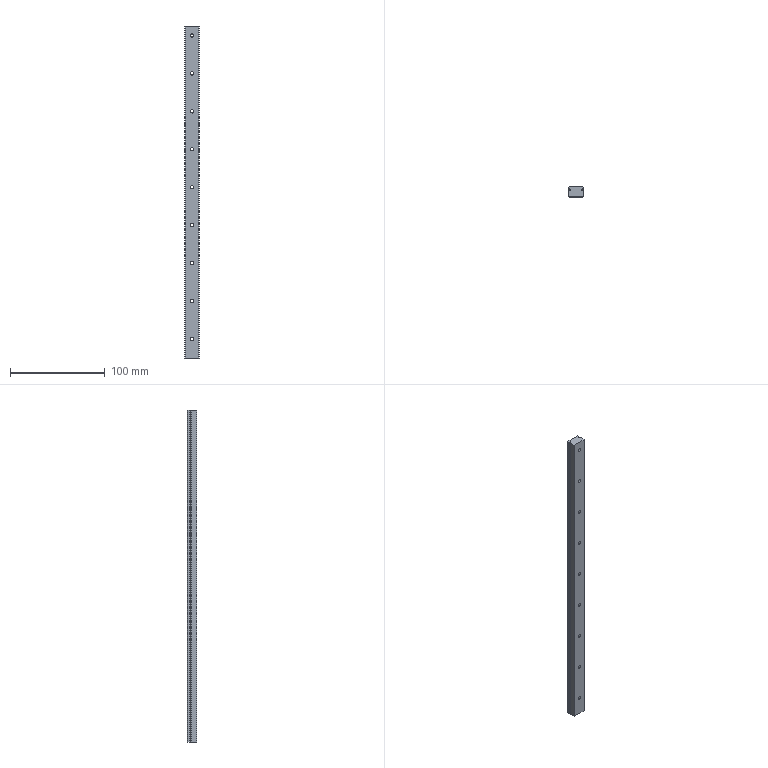Part | SolidWorks | features ICE 18, MirrorSolid 4, Extrusion 3, Fillet 3, MirrorPattern 3, RevCut 3, Chamfer 2, Dome 2, DeleteBody 1, LPattern 1, LibraryFeature 1 | 1 solid | 71 faces | box 15 x 10 x 350 mm | volume 49374 mm3 | cylinder 44 | plane 27 | commonest cylinder face diameters 3.5 x18 6 x18 0.3 x4 2.372 x4